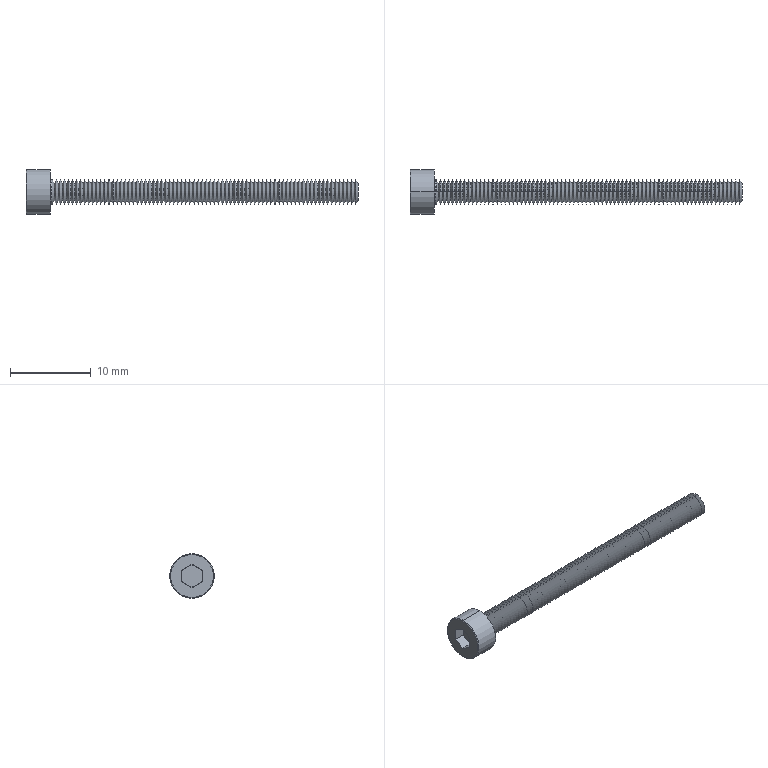Part | SolidWorks | features BaseBody 1 | 1 solid | 494 faces | box 41 x 5.5 x 5.5 mm | volume 259.671 mm3 | cone 318 | cylinder 162 | plane 10 | torus 4 | commonest cylinder face diameters 3 x160 5.5 x2